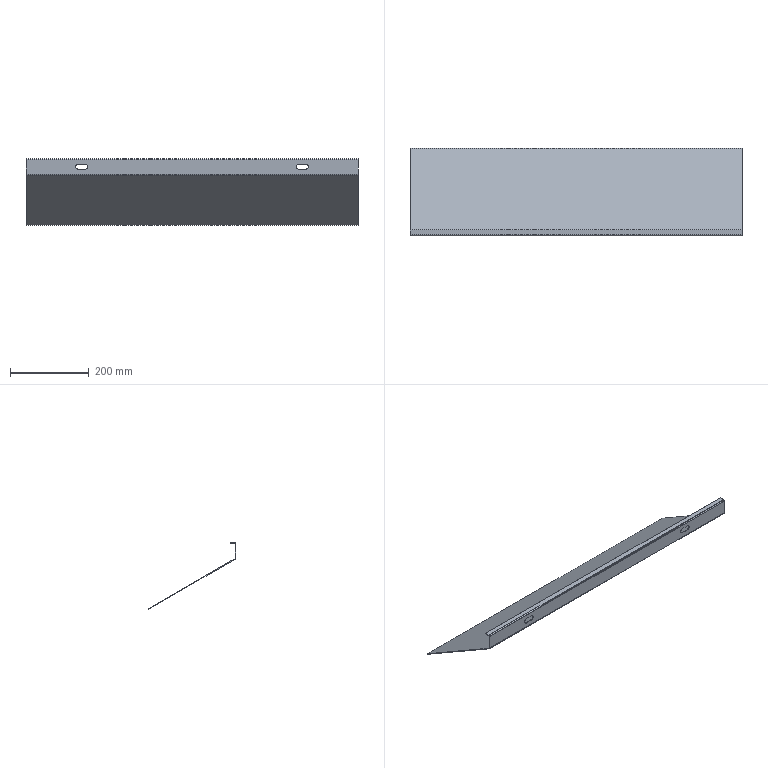Part | SolidWorks | features BaseBody 1 | 1 solid | 22 faces | box 845 x 223.5 x 169.471 mm | volume 391233 mm3 | plane 14 | cylinder 8 | commonest cylinder face diameters 13 x4 3 x2 6 x2
STEP:
#1=CARTESIAN_POINT('',(0.,221.25,-169.471));
#2=VERTEX_POINT('',#1);
#3=CARTESIAN_POINT('',(0.,0.,-41.732));
#4=VERTEX_POINT('',#3);
#5=CARTESIAN_POINT('',(0.,92.7,-95.252));
#6=DIRECTION('',(0.,-0.866,0.5));
#7=VECTOR('',#6,1000.);
#8=LINE('',#5,#7);
#9=EDGE_CURVE('',#2,#4,#8,.T.);
#10=ORIENTED_EDGE('',*,*,#9,.F.);
#11=CARTESIAN_POINT('',(845.,221.25,-169.471));
#12=VERTEX_POINT('',#11);
#13=CARTESIAN_POINT('',(422.5,221.25,-169.471));
#14=DIRECTION('',(-1.,0.,0.));
#15=VECTOR('',#14,1000.);
#16=LINE('',#13,#15);
#17=EDGE_CURVE('',#12,#2,#16,.T.);
#18=ORIENTED_EDGE('',*,*,#17,.F.);
#19=CARTESIAN_POINT('',(845.,0.,-41.732));
#20=VERTEX_POINT('',#19);
#21=CARTESIAN_POINT('',(845.,92.7,-95.252));
#22=DIRECTION('',(0.,0.866,-0.5));
#23=VECTOR('',#22,1000.);
#24=LINE('',#21,#23);
#25=EDGE_CURVE('',#20,#12,#24,.T.);
#26=ORIENTED_EDGE('',*,*,#25,.F.);
#27=CARTESIAN_POINT('',(422.5,0.,-41.732));
#28=DIRECTION('',(1.,0.,0.));
#29=VECTOR('',#28,1000.);
#30=LINE('',#27,#29);
#31=EDGE_CURVE('',#4,#20,#30,.T.);
#32=ORIENTED_EDGE('',*,*,#31,.F.);
#33=EDGE_LOOP('',(#10,#18,#26,#32));
#34=FACE_OUTER_BOUND('',#33,.T.);
#35=CARTESIAN_POINT('',(422.5,92.7,-95.252));
#36=DIRECTION('',(0.,0.5,0.866));
#37=DIRECTION('',(0.,-0.866,0.5));
#38=AXIS2_PLACEMENT_3D('',#35,#36,#37);
#39=PLANE('',#38);
#40=ADVANCED_FACE('',(#34),#39,.F.);
#41=CARTESIAN_POINT('',(845.,-1.5,-39.134));
#42=VERTEX_POINT('',#41);
#43=CARTESIAN_POINT('',(0.,-1.5,-39.134));
#44=VERTEX_POINT('',#43);
#45=CARTESIAN_POINT('',(422.5,-1.5,-39.134));
#46=DIRECTION('',(-1.,0.,0.));
#47=VECTOR('',#46,1000.);
#48=LINE('',#45,#47);
#49=EDGE_CURVE('',#42,#44,#48,.T.);
#50=ORIENTED_EDGE('',*,*,#49,.T.);
#51=CARTESIAN_POINT('',(0.,1.5,-39.134));
#52=DIRECTION('',(1.,0.,0.));
#53=DIRECTION('',(0.,0.,-1.));
#54=AXIS2_PLACEMENT_3D('',#51,#52,#53);
#55=CIRCLE('',#54,3.);
#56=EDGE_CURVE('',#44,#4,#55,.T.);
#57=ORIENTED_EDGE('',*,*,#56,.T.);
#58=ORIENTED_EDGE('',*,*,#31,.T.);
#59=CARTESIAN_POINT('',(845.,1.5,-39.134));
#60=DIRECTION('',(-1.,0.,0.));
#61=DIRECTION('',(0.,0.,-1.));
#62=AXIS2_PLACEMENT_3D('',#59,#60,#61);
#63=CIRCLE('',#62,3.);
#64=EDGE_CURVE('',#20,#42,#63,.T.);
#65=ORIENTED_EDGE('',*,*,#64,.T.);
#66=EDGE_LOOP('',(#50,#57,#58,#65));
#67=FACE_OUTER_BOUND('',#66,.T.);
#68=CARTESIAN_POINT('',(422.5,1.5,-39.134));
#69=DIRECTION('',(1.,0.,0.));
#70=DIRECTION('',(0.,0.,-1.));
#71=AXIS2_PLACEMENT_3D('',#68,#69,#70);
#72=CYLINDRICAL_SURFACE('',#71,3.);
#73=ADVANCED_FACE('',(#67),#72,.T.);
#74=CARTESIAN_POINT('',(0.,222.,-168.172));
#75=VERTEX_POINT('',#74);
#76=CARTESIAN_POINT('',(0.,222.,-168.172));
#77=DIRECTION('',(0.,-0.5,-0.866));
#78=VECTOR('',#77,1000.);
#79=LINE('',#76,#78);
#80=EDGE_CURVE('',#75,#2,#79,.T.);
#81=ORIENTED_EDGE('',*,*,#80,.T.);
#82=ORIENTED_EDGE('',*,*,#9,.T.);
#83=ORIENTED_EDGE('',*,*,#56,.F.);
#84=CARTESIAN_POINT('',(0.,-1.5,-3.));
#85=VERTEX_POINT('',#84);
#86=CARTESIAN_POINT('',(0.,-1.5,-148.437));
#87=DIRECTION('',(0.,0.,1.));
#88=VECTOR('',#87,1000.);
#89=LINE('',#86,#88);
#90=EDGE_CURVE('',#44,#85,#89,.T.);
#91=ORIENTED_EDGE('',*,*,#90,.T.);
#92=CARTESIAN_POINT('',(0.,1.5,0.));
#93=VERTEX_POINT('',#92);
#94=CARTESIAN_POINT('',(0.,1.5,-3.));
#95=DIRECTION('',(1.,0.,0.));
#96=DIRECTION('',(0.,-1.,0.));
#97=AXIS2_PLACEMENT_3D('',#94,#95,#96);
#98=CIRCLE('',#97,3.);
#99=EDGE_CURVE('',#93,#85,#98,.T.);
#100=ORIENTED_EDGE('',*,*,#99,.F.);
#101=CARTESIAN_POINT('',(0.,13.5,0.));
#102=VERTEX_POINT('',#101);
#103=CARTESIAN_POINT('',(0.,5.804,0.));
#104=DIRECTION('',(0.,1.,0.));
#105=VECTOR('',#104,1000.);
#106=LINE('',#103,#105);
#107=EDGE_CURVE('',#93,#102,#106,.T.);
#108=ORIENTED_EDGE('',*,*,#107,.T.);
#109=CARTESIAN_POINT('',(0.,13.5,-1.5));
#110=VERTEX_POINT('',#109);
#111=CARTESIAN_POINT('',(0.,13.5,-1.5));
#112=DIRECTION('',(0.,0.,1.));
#113=VECTOR('',#112,1000.);
#114=LINE('',#111,#113);
#115=EDGE_CURVE('',#110,#102,#114,.T.);
#116=ORIENTED_EDGE('',*,*,#115,.F.);
#117=CARTESIAN_POINT('',(0.,1.5,-1.5));
#118=VERTEX_POINT('',#117);
#119=CARTESIAN_POINT('',(0.,1.5,-1.5));
#120=DIRECTION('',(0.,-1.,0.));
#121=VECTOR('',#120,1000.);
#122=LINE('',#119,#121);
#123=EDGE_CURVE('',#110,#118,#122,.T.);
#124=ORIENTED_EDGE('',*,*,#123,.T.);
#125=CARTESIAN_POINT('',(0.,0.,-3.));
#126=VERTEX_POINT('',#125);
#127=CARTESIAN_POINT('',(0.,1.5,-3.));
#128=DIRECTION('',(1.,0.,0.));
#129=DIRECTION('',(0.,-1.,0.));
#130=AXIS2_PLACEMENT_3D('',#127,#128,#129);
#131=CIRCLE('',#130,1.5);
#132=EDGE_CURVE('',#118,#126,#131,.T.);
#133=ORIENTED_EDGE('',*,*,#132,.T.);
#134=CARTESIAN_POINT('',(0.,0.,-39.134));
#135=VERTEX_POINT('',#134);
#136=CARTESIAN_POINT('',(0.,0.,-41.396));
#137=DIRECTION('',(0.,0.,-1.));
#138=VECTOR('',#137,1000.);
#139=LINE('',#136,#138);
#140=EDGE_CURVE('',#126,#135,#139,.T.);
#141=ORIENTED_EDGE('',*,*,#140,.T.);
#142=CARTESIAN_POINT('',(0.,0.75,-40.433));
#143=VERTEX_POINT('',#142);
#144=CARTESIAN_POINT('',(0.,1.5,-39.134));
#145=DIRECTION('',(1.,0.,0.));
#146=DIRECTION('',(0.,0.,-1.));
#147=AXIS2_PLACEMENT_3D('',#144,#145,#146);
#148=CIRCLE('',#147,1.5);
#149=EDGE_CURVE('',#135,#143,#148,.T.);
#150=ORIENTED_EDGE('',*,*,#149,.T.);
#151=CARTESIAN_POINT('',(0.,0.75,-40.433));
#152=DIRECTION('',(0.,0.866,-0.5));
#153=VECTOR('',#152,1000.);
#154=LINE('',#151,#153);
#155=EDGE_CURVE('',#143,#75,#154,.T.);
#156=ORIENTED_EDGE('',*,*,#155,.T.);
#157=EDGE_LOOP('',(#81,#82,#83,#91,#100,#108,#116,#124,#133,#141,#150,#156));
#158=FACE_OUTER_BOUND('',#157,.T.);
#159=CARTESIAN_POINT('',(0.,0.,-41.732));
#160=DIRECTION('',(-1.,0.,0.));
#161=DIRECTION('',(0.,0.,1.));
#162=AXIS2_PLACEMENT_3D('',#159,#160,#161);
#163=PLANE('',#162);
#164=ADVANCED_FACE('',(#158),#163,.T.);
#165=ORIENTED_EDGE('',*,*,#17,.T.);
#166=ORIENTED_EDGE('',*,*,#80,.F.);
#167=CARTESIAN_POINT('',(845.,222.,-168.172));
#168=VERTEX_POINT('',#167);
#169=CARTESIAN_POINT('',(0.,222.,-168.172));
#170=DIRECTION('',(1.,0.,0.));
#171=VECTOR('',#170,1000.);
#172=LINE('',#169,#171);
#173=EDGE_CURVE('',#75,#168,#172,.T.);
#174=ORIENTED_EDGE('',*,*,#173,.T.);
#175=CARTESIAN_POINT('',(845.,221.25,-169.471));
#176=DIRECTION('',(0.,-0.5,-0.866));
#177=VECTOR('',#176,1000.);
#178=LINE('',#175,#177);
#179=EDGE_CURVE('',#168,#12,#178,.T.);
#180=ORIENTED_EDGE('',*,*,#179,.T.);
#181=EDGE_LOOP('',(#165,#166,#174,#180));
#182=FACE_OUTER_BOUND('',#181,.T.);
#183=CARTESIAN_POINT('',(0.,221.25,-169.471));
#184=DIRECTION('',(0.,0.866,-0.5));
#185=DIRECTION('',(0.,0.5,0.866));
#186=AXIS2_PLACEMENT_3D('',#183,#184,#185);
#187=PLANE('',#186);
#188=ADVANCED_FACE('',(#182),#187,.T.);
#189=ORIENTED_EDGE('',*,*,#179,.F.);
#190=CARTESIAN_POINT('',(845.,0.75,-40.433));
#191=VERTEX_POINT('',#190);
#192=CARTESIAN_POINT('',(845.,222.,-168.172));
#193=DIRECTION('',(0.,-0.866,0.5));
#194=VECTOR('',#193,1000.);
#195=LINE('',#192,#194);
#196=EDGE_CURVE('',#168,#191,#195,.T.);
#197=ORIENTED_EDGE('',*,*,#196,.T.);
#198=CARTESIAN_POINT('',(845.,0.,-39.134));
#199=VERTEX_POINT('',#198);
#200=CARTESIAN_POINT('',(845.,1.5,-39.134));
#201=DIRECTION('',(-1.,0.,0.));
#202=DIRECTION('',(0.,0.,-1.));
#203=AXIS2_PLACEMENT_3D('',#200,#201,#202);
#204=CIRCLE('',#203,1.5);
#205=EDGE_CURVE('',#191,#199,#204,.T.);
#206=ORIENTED_EDGE('',*,*,#205,.T.);
#207=CARTESIAN_POINT('',(845.,0.,-3.));
#208=VERTEX_POINT('',#207);
#209=CARTESIAN_POINT('',(845.,0.,-39.134));
#210=DIRECTION('',(0.,0.,1.));
#211=VECTOR('',#210,1000.);
#212=LINE('',#209,#211);
#213=EDGE_CURVE('',#199,#208,#212,.T.);
#214=ORIENTED_EDGE('',*,*,#213,.T.);
#215=CARTESIAN_POINT('',(845.,1.5,-1.5));
#216=VERTEX_POINT('',#215);
#217=CARTESIAN_POINT('',(845.,1.5,-3.));
#218=DIRECTION('',(-1.,0.,0.));
#219=DIRECTION('',(0.,-1.,0.));
#220=AXIS2_PLACEMENT_3D('',#217,#218,#219);
#221=CIRCLE('',#220,1.5);
#222=EDGE_CURVE('',#208,#216,#221,.T.);
#223=ORIENTED_EDGE('',*,*,#222,.T.);
#224=CARTESIAN_POINT('',(845.,13.5,-1.5));
#225=VERTEX_POINT('',#224);
#226=CARTESIAN_POINT('',(845.,1.5,-1.5));
#227=DIRECTION('',(0.,1.,0.));
#228=VECTOR('',#227,1000.);
#229=LINE('',#226,#228);
#230=EDGE_CURVE('',#216,#225,#229,.T.);
#231=ORIENTED_EDGE('',*,*,#230,.T.);
#232=CARTESIAN_POINT('',(845.,13.5,0.));
#233=VERTEX_POINT('',#232);
#234=CARTESIAN_POINT('',(845.,13.5,-1.5));
#235=DIRECTION('',(0.,0.,1.));
#236=VECTOR('',#235,1000.);
#237=LINE('',#234,#236);
#238=EDGE_CURVE('',#225,#233,#237,.T.);
#239=ORIENTED_EDGE('',*,*,#238,.T.);
#240=CARTESIAN_POINT('',(845.,1.5,0.));
#241=VERTEX_POINT('',#240);
#242=CARTESIAN_POINT('',(845.,5.804,0.));
#243=DIRECTION('',(0.,-1.,0.));
#244=VECTOR('',#243,1000.);
#245=LINE('',#242,#244);
#246=EDGE_CURVE('',#233,#241,#245,.T.);
#247=ORIENTED_EDGE('',*,*,#246,.T.);
#248=CARTESIAN_POINT('',(845.,-1.5,-3.));
#249=VERTEX_POINT('',#248);
#250=CARTESIAN_POINT('',(845.,1.5,-3.));
#251=DIRECTION('',(-1.,0.,0.));
#252=DIRECTION('',(0.,-1.,0.));
#253=AXIS2_PLACEMENT_3D('',#250,#251,#252);
#254=CIRCLE('',#253,3.);
#255=EDGE_CURVE('',#249,#241,#254,.T.);
#256=ORIENTED_EDGE('',*,*,#255,.F.);
#257=CARTESIAN_POINT('',(845.,-1.5,-148.437));
#258=DIRECTION('',(0.,0.,-1.));
#259=VECTOR('',#258,1000.);
#260=LINE('',#257,#259);
#261=EDGE_CURVE('',#249,#42,#260,.T.);
#262=ORIENTED_EDGE('',*,*,#261,.T.);
#263=ORIENTED_EDGE('',*,*,#64,.F.);
#264=ORIENTED_EDGE('',*,*,#25,.T.);
#265=EDGE_LOOP('',(#189,#197,#206,#214,#223,#231,#239,#247,#256,#262,#263,#264));
#266=FACE_OUTER_BOUND('',#265,.T.);
#267=CARTESIAN_POINT('',(845.,-1.959,-40.601));
#268=DIRECTION('',(1.,0.,0.));
#269=DIRECTION('',(0.,0.,-1.));
#270=AXIS2_PLACEMENT_3D('',#267,#268,#269);
#271=PLANE('',#270);
#272=ADVANCED_FACE('',(#266),#271,.T.);
#273=CARTESIAN_POINT('',(695.,-1.5,-26.5));
#274=VERTEX_POINT('',#273);
#275=CARTESIAN_POINT('',(712.,-1.5,-26.5));
#276=VERTEX_POINT('',#275);
#277=CARTESIAN_POINT('',(422.5,-1.5,-26.5));
#278=DIRECTION('',(1.,0.,0.));
#279=VECTOR('',#278,1000.);
#280=LINE('',#277,#279);
#281=EDGE_CURVE('',#274,#276,#280,.T.);
#282=ORIENTED_EDGE('',*,*,#281,.F.);
#283=CARTESIAN_POINT('',(695.,-1.5,-13.5));
#284=VERTEX_POINT('',#283);
#285=CARTESIAN_POINT('',(695.,-1.5,-20.));
#286=DIRECTION('',(0.,-1.,0.));
#287=DIRECTION('',(0.,0.,1.));
#288=AXIS2_PLACEMENT_3D('',#285,#286,#287);
#289=CIRCLE('',#288,6.5);
#290=EDGE_CURVE('',#284,#274,#289,.T.);
#291=ORIENTED_EDGE('',*,*,#290,.F.);
#292=CARTESIAN_POINT('',(712.,-1.5,-13.5));
#293=VERTEX_POINT('',#292);
#294=CARTESIAN_POINT('',(422.5,-1.5,-13.5));
#295=DIRECTION('',(-1.,0.,0.));
#296=VECTOR('',#295,1000.);
#297=LINE('',#294,#296);
#298=EDGE_CURVE('',#293,#284,#297,.T.);
#299=ORIENTED_EDGE('',*,*,#298,.F.);
#300=CARTESIAN_POINT('',(712.,-1.5,-20.));
#301=DIRECTION('',(0.,-1.,0.));
#302=DIRECTION('',(0.,0.,1.));
#303=AXIS2_PLACEMENT_3D('',#300,#301,#302);
#304=CIRCLE('',#303,6.5);
#305=EDGE_CURVE('',#276,#293,#304,.T.);
#306=ORIENTED_EDGE('',*,*,#305,.F.);
#307=EDGE_LOOP('',(#282,#291,#299,#306));
#308=FACE_BOUND('',#307,.T.);
#309=CARTESIAN_POINT('',(133.,-1.5,-26.5));
#310=VERTEX_POINT('',#309);
#311=CARTESIAN_POINT('',(150.,-1.5,-26.5));
#312=VERTEX_POINT('',#311);
#313=CARTESIAN_POINT('',(422.5,-1.5,-26.5));
#314=DIRECTION('',(1.,0.,0.));
#315=VECTOR('',#314,1000.);
#316=LINE('',#313,#315);
#317=EDGE_CURVE('',#310,#312,#316,.T.);
#318=ORIENTED_EDGE('',*,*,#317,.F.);
#319=CARTESIAN_POINT('',(133.,-1.5,-13.5));
#320=VERTEX_POINT('',#319);
#321=CARTESIAN_POINT('',(133.,-1.5,-20.));
#322=DIRECTION('',(0.,-1.,0.));
#323=DIRECTION('',(0.,0.,1.));
#324=AXIS2_PLACEMENT_3D('',#321,#322,#323);
#325=CIRCLE('',#324,6.5);
#326=EDGE_CURVE('',#320,#310,#325,.T.);
#327=ORIENTED_EDGE('',*,*,#326,.F.);
#328=CARTESIAN_POINT('',(150.,-1.5,-13.5));
#329=VERTEX_POINT('',#328);
#330=CARTESIAN_POINT('',(422.5,-1.5,-13.5));
#331=DIRECTION('',(-1.,0.,0.));
#332=VECTOR('',#331,1000.);
#333=LINE('',#330,#332);
#334=EDGE_CURVE('',#329,#320,#333,.T.);
#335=ORIENTED_EDGE('',*,*,#334,.F.);
#336=CARTESIAN_POINT('',(150.,-1.5,-20.));
#337=DIRECTION('',(0.,-1.,0.));
#338=DIRECTION('',(0.,0.,1.));
#339=AXIS2_PLACEMENT_3D('',#336,#337,#338);
#340=CIRCLE('',#339,6.5);
#341=EDGE_CURVE('',#312,#329,#340,.T.);
#342=ORIENTED_EDGE('',*,*,#341,.F.);
#343=EDGE_LOOP('',(#318,#327,#335,#342));
#344=FACE_BOUND('',#343,.T.);
#345=ORIENTED_EDGE('',*,*,#90,.F.);
#346=ORIENTED_EDGE('',*,*,#49,.F.);
#347=ORIENTED_EDGE('',*,*,#261,.F.);
#348=CARTESIAN_POINT('',(422.5,-1.5,-3.));
#349=DIRECTION('',(1.,0.,0.));
#350=VECTOR('',#349,1000.);
#351=LINE('',#348,#350);
#352=EDGE_CURVE('',#85,#249,#351,.T.);
#353=ORIENTED_EDGE('',*,*,#352,.F.);
#354=EDGE_LOOP('',(#345,#346,#347,#353));
#355=FACE_OUTER_BOUND('',#354,.T.);
#356=CARTESIAN_POINT('',(422.5,-1.5,-148.437));
#357=DIRECTION('',(0.,1.,0.));
#358=DIRECTION('',(0.,0.,1.));
#359=AXIS2_PLACEMENT_3D('',#356,#357,#358);
#360=PLANE('',#359);
#361=ADVANCED_FACE('',(#308,#344,#355),#360,.F.);
#362=ORIENTED_EDGE('',*,*,#173,.F.);
#363=ORIENTED_EDGE('',*,*,#155,.F.);
#364=CARTESIAN_POINT('',(422.5,0.75,-40.433));
#365=DIRECTION('',(1.,0.,0.));
#366=VECTOR('',#365,1000.);
#367=LINE('',#364,#366);
#368=EDGE_CURVE('',#143,#191,#367,.T.);
#369=ORIENTED_EDGE('',*,*,#368,.T.);
#370=ORIENTED_EDGE('',*,*,#196,.F.);
#371=EDGE_LOOP('',(#362,#363,#369,#370));
#372=FACE_OUTER_BOUND('',#371,.T.);
#373=CARTESIAN_POINT('',(422.5,93.45,-93.953));
#374=DIRECTION('',(0.,0.5,0.866));
#375=DIRECTION('',(0.,-0.866,0.5));
#376=AXIS2_PLACEMENT_3D('',#373,#374,#375);
#377=PLANE('',#376);
#378=ADVANCED_FACE('',(#372),#377,.T.);
#379=CARTESIAN_POINT('',(712.,0.,-26.5));
#380=VERTEX_POINT('',#379);
#381=CARTESIAN_POINT('',(712.,-1.5,-26.5));
#382=DIRECTION('',(0.,1.,0.));
#383=VECTOR('',#382,1000.);
#384=LINE('',#381,#383);
#385=EDGE_CURVE('',#276,#380,#384,.T.);
#386=ORIENTED_EDGE('',*,*,#385,.F.);
#387=ORIENTED_EDGE('',*,*,#305,.T.);
#388=CARTESIAN_POINT('',(712.,0.,-13.5));
#389=VERTEX_POINT('',#388);
#390=CARTESIAN_POINT('',(712.,-1.5,-13.5));
#391=DIRECTION('',(0.,-1.,0.));
#392=VECTOR('',#391,1000.);
#393=LINE('',#390,#392);
#394=EDGE_CURVE('',#389,#293,#393,.T.);
#395=ORIENTED_EDGE('',*,*,#394,.F.);
#396=CARTESIAN_POINT('',(712.,0.,-20.));
#397=DIRECTION('',(0.,-1.,0.));
#398=DIRECTION('',(0.,0.,1.));
#399=AXIS2_PLACEMENT_3D('',#396,#397,#398);
#400=CIRCLE('',#399,6.5);
#401=EDGE_CURVE('',#380,#389,#400,.T.);
#402=ORIENTED_EDGE('',*,*,#401,.F.);
#403=EDGE_LOOP('',(#386,#387,#395,#402));
#404=FACE_OUTER_BOUND('',#403,.T.);
#405=CARTESIAN_POINT('',(712.,-1.5,-20.));
#406=DIRECTION('',(0.,1.,0.));
#407=DIRECTION('',(0.,0.,1.));
#408=AXIS2_PLACEMENT_3D('',#405,#406,#407);
#409=CYLINDRICAL_SURFACE('',#408,6.5);
#410=ADVANCED_FACE('',(#404),#409,.F.);
#411=CARTESIAN_POINT('',(695.,0.,-26.5));
#412=VERTEX_POINT('',#411);
#413=CARTESIAN_POINT('',(695.,-1.5,-26.5));
#414=DIRECTION('',(0.,1.,0.));
#415=VECTOR('',#414,1000.);
#416=LINE('',#413,#415);
#417=EDGE_CURVE('',#274,#412,#416,.T.);
#418=ORIENTED_EDGE('',*,*,#417,.F.);
#419=ORIENTED_EDGE('',*,*,#281,.T.);
#420=ORIENTED_EDGE('',*,*,#385,.T.);
#421=CARTESIAN_POINT('',(712.,0.,-26.5));
#422=DIRECTION('',(1.,0.,0.));
#423=VECTOR('',#422,1000.);
#424=LINE('',#421,#423);
#425=EDGE_CURVE('',#412,#380,#424,.T.);
#426=ORIENTED_EDGE('',*,*,#425,.F.);
#427=EDGE_LOOP('',(#418,#419,#420,#426));
#428=FACE_OUTER_BOUND('',#427,.T.);
#429=CARTESIAN_POINT('',(712.,-1.5,-26.5));
#430=DIRECTION('',(0.,0.,-1.));
#431=DIRECTION('',(-1.,0.,0.));
#432=AXIS2_PLACEMENT_3D('',#429,#430,#431);
#433=PLANE('',#432);
#434=ADVANCED_FACE('',(#428),#433,.F.);
#435=CARTESIAN_POINT('',(695.,0.,-13.5));
#436=VERTEX_POINT('',#435);
#437=CARTESIAN_POINT('',(695.,-1.5,-13.5));
#438=DIRECTION('',(0.,1.,0.));
#439=VECTOR('',#438,1000.);
#440=LINE('',#437,#439);
#441=EDGE_CURVE('',#284,#436,#440,.T.);
#442=ORIENTED_EDGE('',*,*,#441,.F.);
#443=ORIENTED_EDGE('',*,*,#290,.T.);
#444=ORIENTED_EDGE('',*,*,#417,.T.);
#445=CARTESIAN_POINT('',(695.,0.,-20.));
#446=DIRECTION('',(0.,-1.,0.));
#447=DIRECTION('',(0.,0.,1.));
#448=AXIS2_PLACEMENT_3D('',#445,#446,#447);
#449=CIRCLE('',#448,6.5);
#450=EDGE_CURVE('',#436,#412,#449,.T.);
#451=ORIENTED_EDGE('',*,*,#450,.F.);
#452=EDGE_LOOP('',(#442,#443,#444,#451));
#453=FACE_OUTER_BOUND('',#452,.T.);
#454=CARTESIAN_POINT('',(695.,-1.5,-20.));
#455=DIRECTION('',(0.,1.,0.));
#456=DIRECTION('',(0.,0.,1.));
#457=AXIS2_PLACEMENT_3D('',#454,#455,#456);
#458=CYLINDRICAL_SURFACE('',#457,6.5);
#459=ADVANCED_FACE('',(#453),#458,.F.);
#460=ORIENTED_EDGE('',*,*,#394,.T.);
#461=ORIENTED_EDGE('',*,*,#298,.T.);
#462=ORIENTED_EDGE('',*,*,#441,.T.);
#463=CARTESIAN_POINT('',(695.,0.,-13.5));
#464=DIRECTION('',(-1.,0.,0.));
#465=VECTOR('',#464,1000.);
#466=LINE('',#463,#465);
#467=EDGE_CURVE('',#389,#436,#466,.T.);
#468=ORIENTED_EDGE('',*,*,#467,.F.);
#469=EDGE_LOOP('',(#460,#461,#462,#468));
#470=FACE_OUTER_BOUND('',#469,.T.);
#471=CARTESIAN_POINT('',(695.,-1.5,-13.5));
#472=DIRECTION('',(0.,0.,1.));
#473=DIRECTION('',(1.,0.,0.));
#474=AXIS2_PLACEMENT_3D('',#471,#472,#473);
#475=PLANE('',#474);
#476=ADVANCED_FACE('',(#470),#475,.F.);
#477=CARTESIAN_POINT('',(150.,0.,-26.5));
#478=VERTEX_POINT('',#477);
#479=CARTESIAN_POINT('',(150.,-1.5,-26.5));
#480=DIRECTION('',(0.,1.,0.));
#481=VECTOR('',#480,1000.);
#482=LINE('',#479,#481);
#483=EDGE_CURVE('',#312,#478,#482,.T.);
#484=ORIENTED_EDGE('',*,*,#483,.F.);
#485=ORIENTED_EDGE('',*,*,#341,.T.);
#486=CARTESIAN_POINT('',(150.,0.,-13.5));
#487=VERTEX_POINT('',#486);
#488=CARTESIAN_POINT('',(150.,-1.5,-13.5));
#489=DIRECTION('',(0.,-1.,0.));
#490=VECTOR('',#489,1000.);
#491=LINE('',#488,#490);
#492=EDGE_CURVE('',#487,#329,#491,.T.);
#493=ORIENTED_EDGE('',*,*,#492,.F.);
#494=CARTESIAN_POINT('',(150.,0.,-20.));
#495=DIRECTION('',(0.,-1.,0.));
#496=DIRECTION('',(0.,0.,1.));
#497=AXIS2_PLACEMENT_3D('',#494,#495,#496);
#498=CIRCLE('',#497,6.5);
#499=EDGE_CURVE('',#478,#487,#498,.T.);
#500=ORIENTED_EDGE('',*,*,#499,.F.);
#501=EDGE_LOOP('',(#484,#485,#493,#500));
#502=FACE_OUTER_BOUND('',#501,.T.);
#503=CARTESIAN_POINT('',(150.,-1.5,-20.));
#504=DIRECTION('',(0.,1.,0.));
#505=DIRECTION('',(0.,0.,1.));
#506=AXIS2_PLACEMENT_3D('',#503,#504,#505);
#507=CYLINDRICAL_SURFACE('',#506,6.5);
#508=ADVANCED_FACE('',(#502),#507,.F.);
#509=CARTESIAN_POINT('',(133.,0.,-26.5));
#510=VERTEX_POINT('',#509);
#511=CARTESIAN_POINT('',(133.,-1.5,-26.5));
#512=DIRECTION('',(0.,1.,0.));
#513=VECTOR('',#512,1000.);
#514=LINE('',#511,#513);
#515=EDGE_CURVE('',#310,#510,#514,.T.);
#516=ORIENTED_EDGE('',*,*,#515,.F.);
#517=ORIENTED_EDGE('',*,*,#317,.T.);
#518=ORIENTED_EDGE('',*,*,#483,.T.);
#519=CARTESIAN_POINT('',(150.,0.,-26.5));
#520=DIRECTION('',(1.,0.,0.));
#521=VECTOR('',#520,1000.);
#522=LINE('',#519,#521);
#523=EDGE_CURVE('',#510,#478,#522,.T.);
#524=ORIENTED_EDGE('',*,*,#523,.F.);
#525=EDGE_LOOP('',(#516,#517,#518,#524));
#526=FACE_OUTER_BOUND('',#525,.T.);
#527=CARTESIAN_POINT('',(150.,-1.5,-26.5));
#528=DIRECTION('',(0.,0.,-1.));
#529=DIRECTION('',(0.,1.,0.));
#530=AXIS2_PLACEMENT_3D('',#527,#528,#529);
#531=PLANE('',#530);
#532=ADVANCED_FACE('',(#526),#531,.F.);
#533=CARTESIAN_POINT('',(133.,0.,-13.5));
#534=VERTEX_POINT('',#533);
#535=CARTESIAN_POINT('',(133.,-1.5,-13.5));
#536=DIRECTION('',(0.,1.,0.));
#537=VECTOR('',#536,1000.);
#538=LINE('',#535,#537);
#539=EDGE_CURVE('',#320,#534,#538,.T.);
#540=ORIENTED_EDGE('',*,*,#539,.F.);
#541=ORIENTED_EDGE('',*,*,#326,.T.);
#542=ORIENTED_EDGE('',*,*,#515,.T.);
#543=CARTESIAN_POINT('',(133.,0.,-20.));
#544=DIRECTION('',(0.,-1.,0.));
#545=DIRECTION('',(0.,0.,1.));
#546=AXIS2_PLACEMENT_3D('',#543,#544,#545);
#547=CIRCLE('',#546,6.5);
#548=EDGE_CURVE('',#534,#510,#547,.T.);
#549=ORIENTED_EDGE('',*,*,#548,.F.);
#550=EDGE_LOOP('',(#540,#541,#542,#549));
#551=FACE_OUTER_BOUND('',#550,.T.);
#552=CARTESIAN_POINT('',(133.,-1.5,-20.));
#553=DIRECTION('',(0.,1.,0.));
#554=DIRECTION('',(0.,0.,1.));
#555=AXIS2_PLACEMENT_3D('',#552,#553,#554);
#556=CYLINDRICAL_SURFACE('',#555,6.5);
#557=ADVANCED_FACE('',(#551),#556,.F.);
#558=ORIENTED_EDGE('',*,*,#492,.T.);
#559=ORIENTED_EDGE('',*,*,#334,.T.);
#560=ORIENTED_EDGE('',*,*,#539,.T.);
#561=CARTESIAN_POINT('',(133.,0.,-13.5));
#562=DIRECTION('',(-1.,0.,0.));
#563=VECTOR('',#562,1000.);
#564=LINE('',#561,#563);
#565=EDGE_CURVE('',#487,#534,#564,.T.);
#566=ORIENTED_EDGE('',*,*,#565,.F.);
#567=EDGE_LOOP('',(#558,#559,#560,#566));
#568=FACE_OUTER_BOUND('',#567,.T.);
#569=CARTESIAN_POINT('',(133.,-1.5,-13.5));
#570=DIRECTION('',(0.,0.,1.));
#571=DIRECTION('',(0.,-1.,0.));
#572=AXIS2_PLACEMENT_3D('',#569,#570,#571);
#573=PLANE('',#572);
#574=ADVANCED_FACE('',(#568),#573,.F.);
#575=ORIENTED_EDGE('',*,*,#352,.T.);
#576=ORIENTED_EDGE('',*,*,#255,.T.);
#577=CARTESIAN_POINT('',(422.5,1.5,0.));
#578=DIRECTION('',(-1.,0.,0.));
#579=VECTOR('',#578,1000.);
#580=LINE('',#577,#579);
#581=EDGE_CURVE('',#241,#93,#580,.T.);
#582=ORIENTED_EDGE('',*,*,#581,.T.);
#583=ORIENTED_EDGE('',*,*,#99,.T.);
#584=EDGE_LOOP('',(#575,#576,#582,#583));
#585=FACE_OUTER_BOUND('',#584,.T.);
#586=CARTESIAN_POINT('',(422.5,1.5,-3.));
#587=DIRECTION('',(-1.,0.,0.));
#588=DIRECTION('',(0.,-1.,0.));
#589=AXIS2_PLACEMENT_3D('',#586,#587,#588);
#590=CYLINDRICAL_SURFACE('',#589,3.);
#591=ADVANCED_FACE('',(#585),#590,.T.);
#592=ORIENTED_EDGE('',*,*,#149,.F.);
#593=CARTESIAN_POINT('',(422.5,0.,-39.134));
#594=DIRECTION('',(-1.,0.,0.));
#595=VECTOR('',#594,1000.);
#596=LINE('',#593,#595);
#597=EDGE_CURVE('',#199,#135,#596,.T.);
#598=ORIENTED_EDGE('',*,*,#597,.F.);
#599=ORIENTED_EDGE('',*,*,#205,.F.);
#600=ORIENTED_EDGE('',*,*,#368,.F.);
#601=EDGE_LOOP('',(#592,#598,#599,#600));
#602=FACE_OUTER_BOUND('',#601,.T.);
#603=CARTESIAN_POINT('',(422.5,1.5,-39.134));
#604=DIRECTION('',(1.,0.,0.));
#605=DIRECTION('',(0.,0.,-1.));
#606=AXIS2_PLACEMENT_3D('',#603,#604,#605);
#607=CYLINDRICAL_SURFACE('',#606,1.5);
#608=ADVANCED_FACE('',(#602),#607,.F.);
#609=ORIENTED_EDGE('',*,*,#450,.T.);
#610=ORIENTED_EDGE('',*,*,#425,.T.);
#611=ORIENTED_EDGE('',*,*,#401,.T.);
#612=ORIENTED_EDGE('',*,*,#467,.T.);
#613=EDGE_LOOP('',(#609,#610,#611,#612));
#614=FACE_BOUND('',#613,.T.);
#615=ORIENTED_EDGE('',*,*,#548,.T.);
#616=ORIENTED_EDGE('',*,*,#523,.T.);
#617=ORIENTED_EDGE('',*,*,#499,.T.);
#618=ORIENTED_EDGE('',*,*,#565,.T.);
#619=EDGE_LOOP('',(#615,#616,#617,#618));
#620=FACE_BOUND('',#619,.T.);
#621=ORIENTED_EDGE('',*,*,#597,.T.);
#622=ORIENTED_EDGE('',*,*,#140,.F.);
#623=CARTESIAN_POINT('',(422.5,0.,-3.));
#624=DIRECTION('',(1.,0.,0.));
#625=VECTOR('',#624,1000.);
#626=LINE('',#623,#625);
#627=EDGE_CURVE('',#126,#208,#626,.T.);
#628=ORIENTED_EDGE('',*,*,#627,.T.);
#629=ORIENTED_EDGE('',*,*,#213,.F.);
#630=EDGE_LOOP('',(#621,#622,#628,#629));
#631=FACE_OUTER_BOUND('',#630,.T.);
#632=CARTESIAN_POINT('',(422.5,0.,-148.437));
#633=DIRECTION('',(0.,1.,0.));
#634=DIRECTION('',(0.,0.,1.));
#635=AXIS2_PLACEMENT_3D('',#632,#633,#634);
#636=PLANE('',#635);
#637=ADVANCED_FACE('',(#614,#620,#631),#636,.T.);
#638=ORIENTED_EDGE('',*,*,#246,.F.);
#639=CARTESIAN_POINT('',(422.5,13.5,0.));
#640=DIRECTION('',(1.,0.,0.));
#641=VECTOR('',#640,1000.);
#642=LINE('',#639,#641);
#643=EDGE_CURVE('',#102,#233,#642,.T.);
#644=ORIENTED_EDGE('',*,*,#643,.F.);
#645=ORIENTED_EDGE('',*,*,#107,.F.);
#646=ORIENTED_EDGE('',*,*,#581,.F.);
#647=EDGE_LOOP('',(#638,#644,#645,#646));
#648=FACE_OUTER_BOUND('',#647,.T.);
#649=CARTESIAN_POINT('',(422.5,5.804,0.));
#650=DIRECTION('',(0.,0.,-1.));
#651=DIRECTION('',(0.,1.,0.));
#652=AXIS2_PLACEMENT_3D('',#649,#650,#651);
#653=PLANE('',#652);
#654=ADVANCED_FACE('',(#648),#653,.F.);
#655=ORIENTED_EDGE('',*,*,#222,.F.);
#656=ORIENTED_EDGE('',*,*,#627,.F.);
#657=ORIENTED_EDGE('',*,*,#132,.F.);
#658=CARTESIAN_POINT('',(422.5,1.5,-1.5));
#659=DIRECTION('',(-1.,0.,0.));
#660=VECTOR('',#659,1000.);
#661=LINE('',#658,#660);
#662=EDGE_CURVE('',#216,#118,#661,.T.);
#663=ORIENTED_EDGE('',*,*,#662,.F.);
#664=EDGE_LOOP('',(#655,#656,#657,#663));
#665=FACE_OUTER_BOUND('',#664,.T.);
#666=CARTESIAN_POINT('',(422.5,1.5,-3.));
#667=DIRECTION('',(-1.,0.,0.));
#668=DIRECTION('',(0.,-1.,0.));
#669=AXIS2_PLACEMENT_3D('',#666,#667,#668);
#670=CYLINDRICAL_SURFACE('',#669,1.5);
#671=ADVANCED_FACE('',(#665),#670,.F.);
#672=CARTESIAN_POINT('',(0.,13.5,-1.5));
#673=DIRECTION('',(-1.,0.,0.));
#674=VECTOR('',#673,1000.);
#675=LINE('',#672,#674);
#676=EDGE_CURVE('',#225,#110,#675,.T.);
#677=ORIENTED_EDGE('',*,*,#676,.T.);
#678=ORIENTED_EDGE('',*,*,#115,.T.);
#679=ORIENTED_EDGE('',*,*,#643,.T.);
#680=ORIENTED_EDGE('',*,*,#238,.F.);
#681=EDGE_LOOP('',(#677,#678,#679,#680));
#682=FACE_OUTER_BOUND('',#681,.T.);
#683=CARTESIAN_POINT('',(0.,13.5,-1.5));
#684=DIRECTION('',(0.,1.,0.));
#685=DIRECTION('',(0.,0.,1.));
#686=AXIS2_PLACEMENT_3D('',#683,#684,#685);
#687=PLANE('',#686);
#688=ADVANCED_FACE('',(#682),#687,.T.);
#689=ORIENTED_EDGE('',*,*,#676,.F.);
#690=ORIENTED_EDGE('',*,*,#230,.F.);
#691=ORIENTED_EDGE('',*,*,#662,.T.);
#692=ORIENTED_EDGE('',*,*,#123,.F.);
#693=EDGE_LOOP('',(#689,#690,#691,#692));
#694=FACE_OUTER_BOUND('',#693,.T.);
#695=CARTESIAN_POINT('',(422.5,5.804,-1.5));
#696=DIRECTION('',(0.,0.,-1.));
#697=DIRECTION('',(0.,1.,0.));
#698=AXIS2_PLACEMENT_3D('',#695,#696,#697);
#699=PLANE('',#698);
#700=ADVANCED_FACE('',(#694),#699,.T.);
#701=CLOSED_SHELL('',(#40,#73,#164,#188,#272,#361,#378,#410,#434,#459,#476,#508,#532,#557,#574,#591,#608,#637,#654,#671,#688,#700));
#702=MANIFOLD_SOLID_BREP('',#701);
#703=CARTESIAN_POINT('',(0.,0.,0.));
#704=DIRECTION('',(0.,0.,1.));
#705=DIRECTION('',(1.,0.,0.));
#706=AXIS2_PLACEMENT_3D('',#703,#704,#705);
#707=(LENGTH_UNIT()NAMED_UNIT(*)SI_UNIT(.MILLI.,.METRE.));
#708=UNCERTAINTY_MEASURE_WITH_UNIT(LENGTH_MEASURE(0.00001),#707,'','');
#709=(NAMED_UNIT(*)PLANE_ANGLE_UNIT()SI_UNIT($,.RADIAN.));
#710=(NAMED_UNIT(*)SI_UNIT($,.STERADIAN.)SOLID_ANGLE_UNIT());
#711=(GEOMETRIC_REPRESENTATION_CONTEXT(3)GLOBAL_UNCERTAINTY_ASSIGNED_CONTEXT((#708))GLOBAL_UNIT_ASSIGNED_CONTEXT((#707,#709,#710))REPRESENTATION_CONTEXT('',''));
#712=ADVANCED_BREP_SHAPE_REPRESENTATION('',(#702,#706),#711);